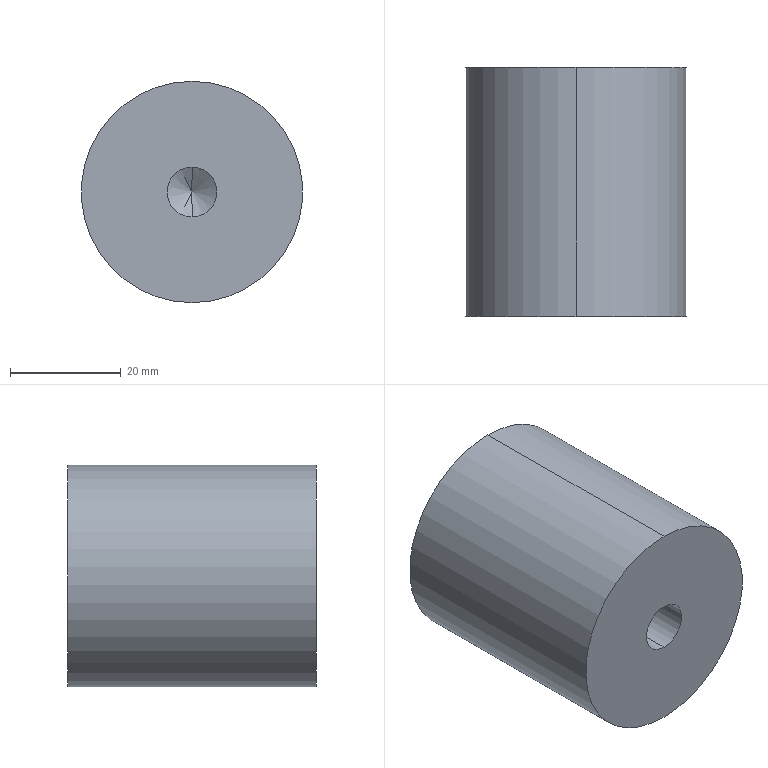Part | STEP file | Microwave Drying Flat Conveyor-silenbloc 40x45xm8 | 1 solid | 12 faces | box 40 x 45 x 40 mm | volume 54907 mm3 | cylinder 6 | cone 4 | plane 2 | commonest cylinder face diameters 9 x4 40 x2
STEP:
#1=CARTESIAN_POINT('',(0.,-10.5,4.5));
#2=VERTEX_POINT('',#1);
#3=CARTESIAN_POINT('',(0.,-10.5,-4.5));
#4=VERTEX_POINT('',#3);
#5=CARTESIAN_POINT('',(0.,-10.5,0.));
#6=DIRECTION('',(0.,-1.,0.));
#7=DIRECTION('',(0.,0.,-1.));
#8=AXIS2_PLACEMENT_3D('',#5,#6,#7);
#9=CIRCLE('',#8,4.5);
#10=EDGE_CURVE('',#2,#4,#9,.T.);
#11=ORIENTED_EDGE('',*,*,#10,.F.);
#12=CARTESIAN_POINT('',(0.,-22.5,4.5));
#13=VERTEX_POINT('',#12);
#14=CARTESIAN_POINT('',(0.,-22.5,4.5));
#15=DIRECTION('',(0.,-1.,0.));
#16=VECTOR('',#15,1000.);
#17=LINE('',#14,#16);
#18=EDGE_CURVE('',#2,#13,#17,.T.);
#19=ORIENTED_EDGE('',*,*,#18,.T.);
#20=CARTESIAN_POINT('',(0.,-22.5,-4.5));
#21=VERTEX_POINT('',#20);
#22=CARTESIAN_POINT('',(0.,-22.5,0.));
#23=DIRECTION('',(0.,-1.,0.));
#24=DIRECTION('',(0.,0.,-1.));
#25=AXIS2_PLACEMENT_3D('',#22,#23,#24);
#26=CIRCLE('',#25,4.5);
#27=EDGE_CURVE('',#13,#21,#26,.T.);
#28=ORIENTED_EDGE('',*,*,#27,.T.);
#29=CARTESIAN_POINT('',(0.,-22.5,-4.5));
#30=DIRECTION('',(0.,-1.,0.));
#31=VECTOR('',#30,1000.);
#32=LINE('',#29,#31);
#33=EDGE_CURVE('',#4,#21,#32,.T.);
#34=ORIENTED_EDGE('',*,*,#33,.F.);
#35=EDGE_LOOP('',(#11,#19,#28,#34));
#36=FACE_OUTER_BOUND('',#35,.T.);
#37=CARTESIAN_POINT('',(0.,-22.5,0.));
#38=DIRECTION('',(0.,-1.,0.));
#39=DIRECTION('',(0.,0.,-1.));
#40=AXIS2_PLACEMENT_3D('',#37,#38,#39);
#41=CYLINDRICAL_SURFACE('',#40,4.5);
#42=ADVANCED_FACE('',(#36),#41,.F.);
#43=CARTESIAN_POINT('',(0.,-7.796,0.));
#44=VERTEX_POINT('',#43);
#45=CARTESIAN_POINT('',(0.,-10.5,-4.5));
#46=DIRECTION('',(0.,-0.515,-0.8572));
#47=VECTOR('',#46,1000.);
#48=LINE('',#45,#47);
#49=EDGE_CURVE('',#44,#4,#48,.T.);
#50=ORIENTED_EDGE('',*,*,#49,.F.);
#51=CARTESIAN_POINT('',(0.,-10.5,4.5));
#52=DIRECTION('',(0.,-0.515,0.8572));
#53=VECTOR('',#52,1000.);
#54=LINE('',#51,#53);
#55=EDGE_CURVE('',#44,#2,#54,.T.);
#56=ORIENTED_EDGE('',*,*,#55,.T.);
#57=ORIENTED_EDGE('',*,*,#10,.T.);
#58=EDGE_LOOP('',(#50,#56,#57));
#59=FACE_OUTER_BOUND('',#58,.T.);
#60=CARTESIAN_POINT('',(0.,-10.5,0.));
#61=DIRECTION('',(0.,-1.,0.));
#62=DIRECTION('',(0.,0.,-1.));
#63=AXIS2_PLACEMENT_3D('',#60,#61,#62);
#64=CONICAL_SURFACE('',#63,4.5,1.03);
#65=ADVANCED_FACE('',(#59),#64,.F.);
#66=CARTESIAN_POINT('',(0.,10.5,-4.5));
#67=VERTEX_POINT('',#66);
#68=CARTESIAN_POINT('',(0.,10.5,4.5));
#69=VERTEX_POINT('',#68);
#70=CARTESIAN_POINT('',(0.,10.5,0.));
#71=DIRECTION('',(0.,1.,0.));
#72=DIRECTION('',(0.,0.,1.));
#73=AXIS2_PLACEMENT_3D('',#70,#71,#72);
#74=CIRCLE('',#73,4.5);
#75=EDGE_CURVE('',#67,#69,#74,.T.);
#76=ORIENTED_EDGE('',*,*,#75,.F.);
#77=CARTESIAN_POINT('',(0.,22.5,-4.5));
#78=VERTEX_POINT('',#77);
#79=CARTESIAN_POINT('',(0.,22.5,-4.5));
#80=DIRECTION('',(0.,1.,0.));
#81=VECTOR('',#80,1000.);
#82=LINE('',#79,#81);
#83=EDGE_CURVE('',#67,#78,#82,.T.);
#84=ORIENTED_EDGE('',*,*,#83,.T.);
#85=CARTESIAN_POINT('',(0.,22.5,4.5));
#86=VERTEX_POINT('',#85);
#87=CARTESIAN_POINT('',(0.,22.5,0.));
#88=DIRECTION('',(0.,1.,0.));
#89=DIRECTION('',(0.,0.,1.));
#90=AXIS2_PLACEMENT_3D('',#87,#88,#89);
#91=CIRCLE('',#90,4.5);
#92=EDGE_CURVE('',#78,#86,#91,.T.);
#93=ORIENTED_EDGE('',*,*,#92,.T.);
#94=CARTESIAN_POINT('',(0.,22.5,4.5));
#95=DIRECTION('',(0.,1.,0.));
#96=VECTOR('',#95,1000.);
#97=LINE('',#94,#96);
#98=EDGE_CURVE('',#69,#86,#97,.T.);
#99=ORIENTED_EDGE('',*,*,#98,.F.);
#100=EDGE_LOOP('',(#76,#84,#93,#99));
#101=FACE_OUTER_BOUND('',#100,.T.);
#102=CARTESIAN_POINT('',(0.,22.5,0.));
#103=DIRECTION('',(0.,1.,0.));
#104=DIRECTION('',(0.,0.,1.));
#105=AXIS2_PLACEMENT_3D('',#102,#103,#104);
#106=CYLINDRICAL_SURFACE('',#105,4.5);
#107=ADVANCED_FACE('',(#101),#106,.F.);
#108=CARTESIAN_POINT('',(0.,7.796,0.));
#109=VERTEX_POINT('',#108);
#110=CARTESIAN_POINT('',(0.,10.5,4.5));
#111=DIRECTION('',(0.,0.515,0.8572));
#112=VECTOR('',#111,1000.);
#113=LINE('',#110,#112);
#114=EDGE_CURVE('',#109,#69,#113,.T.);
#115=ORIENTED_EDGE('',*,*,#114,.F.);
#116=CARTESIAN_POINT('',(0.,10.5,-4.5));
#117=DIRECTION('',(0.,0.515,-0.8572));
#118=VECTOR('',#117,1000.);
#119=LINE('',#116,#118);
#120=EDGE_CURVE('',#109,#67,#119,.T.);
#121=ORIENTED_EDGE('',*,*,#120,.T.);
#122=ORIENTED_EDGE('',*,*,#75,.T.);
#123=EDGE_LOOP('',(#115,#121,#122));
#124=FACE_OUTER_BOUND('',#123,.T.);
#125=CARTESIAN_POINT('',(0.,10.5,0.));
#126=DIRECTION('',(0.,1.,0.));
#127=DIRECTION('',(0.,0.,1.));
#128=AXIS2_PLACEMENT_3D('',#125,#126,#127);
#129=CONICAL_SURFACE('',#128,4.5,1.03);
#130=ADVANCED_FACE('',(#124),#129,.F.);
#131=CARTESIAN_POINT('',(0.,22.5,20.));
#132=VERTEX_POINT('',#131);
#133=CARTESIAN_POINT('',(0.,22.5,-20.));
#134=VERTEX_POINT('',#133);
#135=CARTESIAN_POINT('',(0.,22.5,0.));
#136=DIRECTION('',(0.,1.,0.));
#137=DIRECTION('',(0.,0.,1.));
#138=AXIS2_PLACEMENT_3D('',#135,#136,#137);
#139=CIRCLE('',#138,20.);
#140=EDGE_CURVE('',#132,#134,#139,.T.);
#141=ORIENTED_EDGE('',*,*,#140,.F.);
#142=CARTESIAN_POINT('',(0.,-22.5,20.));
#143=VERTEX_POINT('',#142);
#144=CARTESIAN_POINT('',(0.,22.5,20.));
#145=DIRECTION('',(0.,-1.,0.));
#146=VECTOR('',#145,1000.);
#147=LINE('',#144,#146);
#148=EDGE_CURVE('',#132,#143,#147,.T.);
#149=ORIENTED_EDGE('',*,*,#148,.T.);
#150=CARTESIAN_POINT('',(0.,-22.5,-20.));
#151=VERTEX_POINT('',#150);
#152=CARTESIAN_POINT('',(0.,-22.5,0.));
#153=DIRECTION('',(0.,1.,0.));
#154=DIRECTION('',(0.,0.,1.));
#155=AXIS2_PLACEMENT_3D('',#152,#153,#154);
#156=CIRCLE('',#155,20.);
#157=EDGE_CURVE('',#143,#151,#156,.T.);
#158=ORIENTED_EDGE('',*,*,#157,.T.);
#159=CARTESIAN_POINT('',(0.,22.5,-20.));
#160=DIRECTION('',(0.,-1.,0.));
#161=VECTOR('',#160,1000.);
#162=LINE('',#159,#161);
#163=EDGE_CURVE('',#134,#151,#162,.T.);
#164=ORIENTED_EDGE('',*,*,#163,.F.);
#165=EDGE_LOOP('',(#141,#149,#158,#164));
#166=FACE_OUTER_BOUND('',#165,.T.);
#167=CARTESIAN_POINT('',(0.,22.5,0.));
#168=DIRECTION('',(0.,-1.,0.));
#169=DIRECTION('',(0.,0.,-1.));
#170=AXIS2_PLACEMENT_3D('',#167,#168,#169);
#171=CYLINDRICAL_SURFACE('',#170,20.);
#172=ADVANCED_FACE('',(#166),#171,.T.);
#173=ORIENTED_EDGE('',*,*,#148,.F.);
#174=CARTESIAN_POINT('',(0.,22.5,0.));
#175=DIRECTION('',(0.,1.,0.));
#176=DIRECTION('',(0.,0.,1.));
#177=AXIS2_PLACEMENT_3D('',#174,#175,#176);
#178=CIRCLE('',#177,20.);
#179=EDGE_CURVE('',#134,#132,#178,.T.);
#180=ORIENTED_EDGE('',*,*,#179,.F.);
#181=ORIENTED_EDGE('',*,*,#163,.T.);
#182=CARTESIAN_POINT('',(0.,-22.5,0.));
#183=DIRECTION('',(0.,1.,0.));
#184=DIRECTION('',(0.,0.,1.));
#185=AXIS2_PLACEMENT_3D('',#182,#183,#184);
#186=CIRCLE('',#185,20.);
#187=EDGE_CURVE('',#151,#143,#186,.T.);
#188=ORIENTED_EDGE('',*,*,#187,.T.);
#189=EDGE_LOOP('',(#173,#180,#181,#188));
#190=FACE_OUTER_BOUND('',#189,.T.);
#191=CARTESIAN_POINT('',(0.,22.5,0.));
#192=DIRECTION('',(0.,-1.,0.));
#193=DIRECTION('',(0.,0.,-1.));
#194=AXIS2_PLACEMENT_3D('',#191,#192,#193);
#195=CYLINDRICAL_SURFACE('',#194,20.);
#196=ADVANCED_FACE('',(#190),#195,.T.);
#197=CARTESIAN_POINT('',(0.,22.5,0.));
#198=DIRECTION('',(0.,1.,0.));
#199=DIRECTION('',(0.,0.,1.));
#200=AXIS2_PLACEMENT_3D('',#197,#198,#199);
#201=CIRCLE('',#200,4.5);
#202=EDGE_CURVE('',#86,#78,#201,.T.);
#203=ORIENTED_EDGE('',*,*,#202,.F.);
#204=ORIENTED_EDGE('',*,*,#92,.F.);
#205=EDGE_LOOP('',(#203,#204));
#206=FACE_BOUND('',#205,.T.);
#207=ORIENTED_EDGE('',*,*,#179,.T.);
#208=ORIENTED_EDGE('',*,*,#140,.T.);
#209=EDGE_LOOP('',(#207,#208));
#210=FACE_OUTER_BOUND('',#209,.T.);
#211=CARTESIAN_POINT('',(0.,22.5,0.));
#212=DIRECTION('',(0.,1.,0.));
#213=DIRECTION('',(0.,0.,1.));
#214=AXIS2_PLACEMENT_3D('',#211,#212,#213);
#215=PLANE('',#214);
#216=ADVANCED_FACE('',(#206,#210),#215,.T.);
#217=CARTESIAN_POINT('',(0.,-22.5,0.));
#218=DIRECTION('',(0.,-1.,0.));
#219=DIRECTION('',(0.,0.,-1.));
#220=AXIS2_PLACEMENT_3D('',#217,#218,#219);
#221=CIRCLE('',#220,4.5);
#222=EDGE_CURVE('',#21,#13,#221,.T.);
#223=ORIENTED_EDGE('',*,*,#222,.F.);
#224=ORIENTED_EDGE('',*,*,#27,.F.);
#225=EDGE_LOOP('',(#223,#224));
#226=FACE_BOUND('',#225,.T.);
#227=ORIENTED_EDGE('',*,*,#187,.F.);
#228=ORIENTED_EDGE('',*,*,#157,.F.);
#229=EDGE_LOOP('',(#227,#228));
#230=FACE_OUTER_BOUND('',#229,.T.);
#231=CARTESIAN_POINT('',(0.,-22.5,0.));
#232=DIRECTION('',(0.,1.,0.));
#233=DIRECTION('',(0.,0.,1.));
#234=AXIS2_PLACEMENT_3D('',#231,#232,#233);
#235=PLANE('',#234);
#236=ADVANCED_FACE('',(#226,#230),#235,.F.);
#237=ORIENTED_EDGE('',*,*,#120,.F.);
#238=ORIENTED_EDGE('',*,*,#114,.T.);
#239=CARTESIAN_POINT('',(0.,10.5,0.));
#240=DIRECTION('',(0.,1.,0.));
#241=DIRECTION('',(0.,0.,1.));
#242=AXIS2_PLACEMENT_3D('',#239,#240,#241);
#243=CIRCLE('',#242,4.5);
#244=EDGE_CURVE('',#69,#67,#243,.T.);
#245=ORIENTED_EDGE('',*,*,#244,.T.);
#246=EDGE_LOOP('',(#237,#238,#245));
#247=FACE_OUTER_BOUND('',#246,.T.);
#248=CARTESIAN_POINT('',(0.,10.5,0.));
#249=DIRECTION('',(0.,1.,0.));
#250=DIRECTION('',(0.,0.,1.));
#251=AXIS2_PLACEMENT_3D('',#248,#249,#250);
#252=CONICAL_SURFACE('',#251,4.5,1.03);
#253=ADVANCED_FACE('',(#247),#252,.F.);
#254=ORIENTED_EDGE('',*,*,#83,.F.);
#255=ORIENTED_EDGE('',*,*,#244,.F.);
#256=ORIENTED_EDGE('',*,*,#98,.T.);
#257=ORIENTED_EDGE('',*,*,#202,.T.);
#258=EDGE_LOOP('',(#254,#255,#256,#257));
#259=FACE_OUTER_BOUND('',#258,.T.);
#260=CARTESIAN_POINT('',(0.,22.5,0.));
#261=DIRECTION('',(0.,1.,0.));
#262=DIRECTION('',(0.,0.,1.));
#263=AXIS2_PLACEMENT_3D('',#260,#261,#262);
#264=CYLINDRICAL_SURFACE('',#263,4.5);
#265=ADVANCED_FACE('',(#259),#264,.F.);
#266=ORIENTED_EDGE('',*,*,#55,.F.);
#267=ORIENTED_EDGE('',*,*,#49,.T.);
#268=CARTESIAN_POINT('',(0.,-10.5,0.));
#269=DIRECTION('',(0.,-1.,0.));
#270=DIRECTION('',(0.,0.,-1.));
#271=AXIS2_PLACEMENT_3D('',#268,#269,#270);
#272=CIRCLE('',#271,4.5);
#273=EDGE_CURVE('',#4,#2,#272,.T.);
#274=ORIENTED_EDGE('',*,*,#273,.T.);
#275=EDGE_LOOP('',(#266,#267,#274));
#276=FACE_OUTER_BOUND('',#275,.T.);
#277=CARTESIAN_POINT('',(0.,-10.5,0.));
#278=DIRECTION('',(0.,-1.,0.));
#279=DIRECTION('',(0.,0.,-1.));
#280=AXIS2_PLACEMENT_3D('',#277,#278,#279);
#281=CONICAL_SURFACE('',#280,4.5,1.03);
#282=ADVANCED_FACE('',(#276),#281,.F.);
#283=ORIENTED_EDGE('',*,*,#18,.F.);
#284=ORIENTED_EDGE('',*,*,#273,.F.);
#285=ORIENTED_EDGE('',*,*,#33,.T.);
#286=ORIENTED_EDGE('',*,*,#222,.T.);
#287=EDGE_LOOP('',(#283,#284,#285,#286));
#288=FACE_OUTER_BOUND('',#287,.T.);
#289=CARTESIAN_POINT('',(0.,-22.5,0.));
#290=DIRECTION('',(0.,-1.,0.));
#291=DIRECTION('',(0.,0.,-1.));
#292=AXIS2_PLACEMENT_3D('',#289,#290,#291);
#293=CYLINDRICAL_SURFACE('',#292,4.5);
#294=ADVANCED_FACE('',(#288),#293,.F.);
#295=CLOSED_SHELL('',(#42,#65,#107,#130,#172,#196,#216,#236,#253,#265,#282,#294));
#296=MANIFOLD_SOLID_BREP('',#295);
#297=CARTESIAN_POINT('',(0.,0.,0.));
#298=DIRECTION('',(0.,0.,1.));
#299=DIRECTION('',(1.,0.,0.));
#300=AXIS2_PLACEMENT_3D('',#297,#298,#299);
#301=(LENGTH_UNIT()NAMED_UNIT(*)SI_UNIT(.MILLI.,.METRE.));
#302=UNCERTAINTY_MEASURE_WITH_UNIT(LENGTH_MEASURE(0.00001),#301,'','');
#303=(NAMED_UNIT(*)PLANE_ANGLE_UNIT()SI_UNIT($,.RADIAN.));
#304=(NAMED_UNIT(*)SI_UNIT($,.STERADIAN.)SOLID_ANGLE_UNIT());
#305=(GEOMETRIC_REPRESENTATION_CONTEXT(3)GLOBAL_UNCERTAINTY_ASSIGNED_CONTEXT((#302))GLOBAL_UNIT_ASSIGNED_CONTEXT((#301,#303,#304))REPRESENTATION_CONTEXT('',''));
#306=ADVANCED_BREP_SHAPE_REPRESENTATION('',(#296,#300),#305);